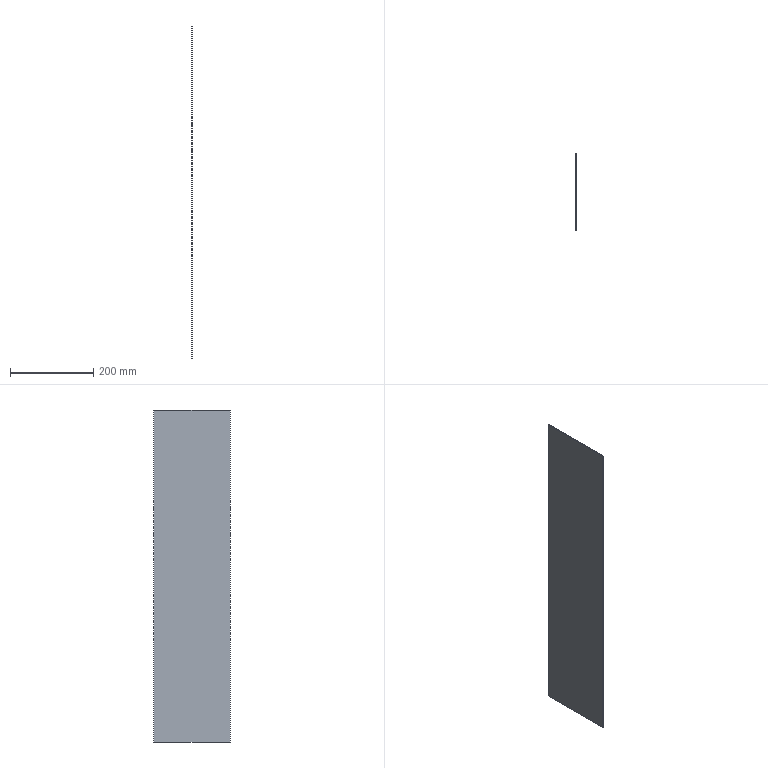Part | SolidWorks | 1 solid | 6 faces | box 1.5 x 185 x 800 mm | volume 222000 mm3 | plane 6
STEP:
#1=CARTESIAN_POINT('',(0.,92.5,400.));
#2=VERTEX_POINT('',#1);
#3=CARTESIAN_POINT('',(0.,-92.5,400.));
#4=VERTEX_POINT('',#3);
#5=CARTESIAN_POINT('',(0.,-92.5,400.));
#6=DIRECTION('',(0.,-1.,0.));
#7=VECTOR('',#6,1000.);
#8=LINE('',#5,#7);
#9=EDGE_CURVE('',#2,#4,#8,.T.);
#10=ORIENTED_EDGE('',*,*,#9,.F.);
#11=CARTESIAN_POINT('',(-1.5,92.5,400.));
#12=VERTEX_POINT('',#11);
#13=CARTESIAN_POINT('',(-1.5,92.5,400.));
#14=DIRECTION('',(1.,0.,0.));
#15=VECTOR('',#14,1000.);
#16=LINE('',#13,#15);
#17=EDGE_CURVE('',#12,#2,#16,.T.);
#18=ORIENTED_EDGE('',*,*,#17,.F.);
#19=CARTESIAN_POINT('',(-1.5,-92.5,400.));
#20=VERTEX_POINT('',#19);
#21=CARTESIAN_POINT('',(-1.5,-92.5,400.));
#22=DIRECTION('',(0.,-1.,0.));
#23=VECTOR('',#22,1000.);
#24=LINE('',#21,#23);
#25=EDGE_CURVE('',#12,#20,#24,.T.);
#26=ORIENTED_EDGE('',*,*,#25,.T.);
#27=CARTESIAN_POINT('',(-1.5,-92.5,400.));
#28=DIRECTION('',(1.,0.,0.));
#29=VECTOR('',#28,1000.);
#30=LINE('',#27,#29);
#31=EDGE_CURVE('',#20,#4,#30,.T.);
#32=ORIENTED_EDGE('',*,*,#31,.T.);
#33=EDGE_LOOP('',(#10,#18,#26,#32));
#34=FACE_OUTER_BOUND('',#33,.T.);
#35=CARTESIAN_POINT('',(-1.5,-92.5,400.));
#36=DIRECTION('',(0.,0.,1.));
#37=DIRECTION('',(1.,0.,0.));
#38=AXIS2_PLACEMENT_3D('',#35,#36,#37);
#39=PLANE('',#38);
#40=ADVANCED_FACE('',(#34),#39,.T.);
#41=CARTESIAN_POINT('',(0.,92.5,-400.));
#42=VERTEX_POINT('',#41);
#43=CARTESIAN_POINT('',(0.,92.5,-400.));
#44=DIRECTION('',(0.,0.,1.));
#45=VECTOR('',#44,1000.);
#46=LINE('',#43,#45);
#47=EDGE_CURVE('',#42,#2,#46,.T.);
#48=ORIENTED_EDGE('',*,*,#47,.F.);
#49=CARTESIAN_POINT('',(-1.5,92.5,-400.));
#50=VERTEX_POINT('',#49);
#51=CARTESIAN_POINT('',(-1.5,92.5,-400.));
#52=DIRECTION('',(1.,0.,0.));
#53=VECTOR('',#52,1000.);
#54=LINE('',#51,#53);
#55=EDGE_CURVE('',#50,#42,#54,.T.);
#56=ORIENTED_EDGE('',*,*,#55,.F.);
#57=CARTESIAN_POINT('',(-1.5,92.5,-400.));
#58=DIRECTION('',(0.,0.,1.));
#59=VECTOR('',#58,1000.);
#60=LINE('',#57,#59);
#61=EDGE_CURVE('',#50,#12,#60,.T.);
#62=ORIENTED_EDGE('',*,*,#61,.T.);
#63=ORIENTED_EDGE('',*,*,#17,.T.);
#64=EDGE_LOOP('',(#48,#56,#62,#63));
#65=FACE_OUTER_BOUND('',#64,.T.);
#66=CARTESIAN_POINT('',(-1.5,92.5,-400.));
#67=DIRECTION('',(0.,1.,0.));
#68=DIRECTION('',(0.,0.,1.));
#69=AXIS2_PLACEMENT_3D('',#66,#67,#68);
#70=PLANE('',#69);
#71=ADVANCED_FACE('',(#65),#70,.T.);
#72=CARTESIAN_POINT('',(0.,-92.5,-400.));
#73=VERTEX_POINT('',#72);
#74=CARTESIAN_POINT('',(0.,-92.5,-400.));
#75=DIRECTION('',(0.,1.,0.));
#76=VECTOR('',#75,1000.);
#77=LINE('',#74,#76);
#78=EDGE_CURVE('',#73,#42,#77,.T.);
#79=ORIENTED_EDGE('',*,*,#78,.F.);
#80=CARTESIAN_POINT('',(-1.5,-92.5,-400.));
#81=VERTEX_POINT('',#80);
#82=CARTESIAN_POINT('',(-1.5,-92.5,-400.));
#83=DIRECTION('',(1.,0.,0.));
#84=VECTOR('',#83,1000.);
#85=LINE('',#82,#84);
#86=EDGE_CURVE('',#81,#73,#85,.T.);
#87=ORIENTED_EDGE('',*,*,#86,.F.);
#88=CARTESIAN_POINT('',(-1.5,-92.5,-400.));
#89=DIRECTION('',(0.,1.,0.));
#90=VECTOR('',#89,1000.);
#91=LINE('',#88,#90);
#92=EDGE_CURVE('',#81,#50,#91,.T.);
#93=ORIENTED_EDGE('',*,*,#92,.T.);
#94=ORIENTED_EDGE('',*,*,#55,.T.);
#95=EDGE_LOOP('',(#79,#87,#93,#94));
#96=FACE_OUTER_BOUND('',#95,.T.);
#97=CARTESIAN_POINT('',(-1.5,-92.5,-400.));
#98=DIRECTION('',(0.,0.,-1.));
#99=DIRECTION('',(-1.,0.,0.));
#100=AXIS2_PLACEMENT_3D('',#97,#98,#99);
#101=PLANE('',#100);
#102=ADVANCED_FACE('',(#96),#101,.T.);
#103=CARTESIAN_POINT('',(0.,-92.5,-400.));
#104=DIRECTION('',(0.,0.,-1.));
#105=VECTOR('',#104,1000.);
#106=LINE('',#103,#105);
#107=EDGE_CURVE('',#4,#73,#106,.T.);
#108=ORIENTED_EDGE('',*,*,#107,.F.);
#109=ORIENTED_EDGE('',*,*,#31,.F.);
#110=CARTESIAN_POINT('',(-1.5,-92.5,-400.));
#111=DIRECTION('',(0.,0.,-1.));
#112=VECTOR('',#111,1000.);
#113=LINE('',#110,#112);
#114=EDGE_CURVE('',#20,#81,#113,.T.);
#115=ORIENTED_EDGE('',*,*,#114,.T.);
#116=ORIENTED_EDGE('',*,*,#86,.T.);
#117=EDGE_LOOP('',(#108,#109,#115,#116));
#118=FACE_OUTER_BOUND('',#117,.T.);
#119=CARTESIAN_POINT('',(-1.5,-92.5,-400.));
#120=DIRECTION('',(0.,-1.,0.));
#121=DIRECTION('',(0.,0.,-1.));
#122=AXIS2_PLACEMENT_3D('',#119,#120,#121);
#123=PLANE('',#122);
#124=ADVANCED_FACE('',(#118),#123,.T.);
#125=ORIENTED_EDGE('',*,*,#25,.F.);
#126=ORIENTED_EDGE('',*,*,#61,.F.);
#127=ORIENTED_EDGE('',*,*,#92,.F.);
#128=ORIENTED_EDGE('',*,*,#114,.F.);
#129=EDGE_LOOP('',(#125,#126,#127,#128));
#130=FACE_OUTER_BOUND('',#129,.T.);
#131=CARTESIAN_POINT('',(-1.5,0.,0.));
#132=DIRECTION('',(1.,0.,0.));
#133=DIRECTION('',(0.,0.,-1.));
#134=AXIS2_PLACEMENT_3D('',#131,#132,#133);
#135=PLANE('',#134);
#136=ADVANCED_FACE('',(#130),#135,.F.);
#137=ORIENTED_EDGE('',*,*,#9,.T.);
#138=ORIENTED_EDGE('',*,*,#107,.T.);
#139=ORIENTED_EDGE('',*,*,#78,.T.);
#140=ORIENTED_EDGE('',*,*,#47,.T.);
#141=EDGE_LOOP('',(#137,#138,#139,#140));
#142=FACE_OUTER_BOUND('',#141,.T.);
#143=CARTESIAN_POINT('',(0.,0.,0.));
#144=DIRECTION('',(1.,0.,0.));
#145=DIRECTION('',(0.,0.,-1.));
#146=AXIS2_PLACEMENT_3D('',#143,#144,#145);
#147=PLANE('',#146);
#148=ADVANCED_FACE('',(#142),#147,.T.);
#149=CLOSED_SHELL('',(#40,#71,#102,#124,#136,#148));
#150=MANIFOLD_SOLID_BREP('',#149);
#151=CARTESIAN_POINT('',(0.,0.,0.));
#152=DIRECTION('',(0.,0.,1.));
#153=DIRECTION('',(1.,0.,0.));
#154=AXIS2_PLACEMENT_3D('',#151,#152,#153);
#155=(LENGTH_UNIT()NAMED_UNIT(*)SI_UNIT(.MILLI.,.METRE.));
#156=UNCERTAINTY_MEASURE_WITH_UNIT(LENGTH_MEASURE(0.00001),#155,'','');
#157=(NAMED_UNIT(*)PLANE_ANGLE_UNIT()SI_UNIT($,.RADIAN.));
#158=(NAMED_UNIT(*)SI_UNIT($,.STERADIAN.)SOLID_ANGLE_UNIT());
#159=(GEOMETRIC_REPRESENTATION_CONTEXT(3)GLOBAL_UNCERTAINTY_ASSIGNED_CONTEXT((#156))GLOBAL_UNIT_ASSIGNED_CONTEXT((#155,#157,#158))REPRESENTATION_CONTEXT('',''));
#160=ADVANCED_BREP_SHAPE_REPRESENTATION('',(#150,#154),#159);